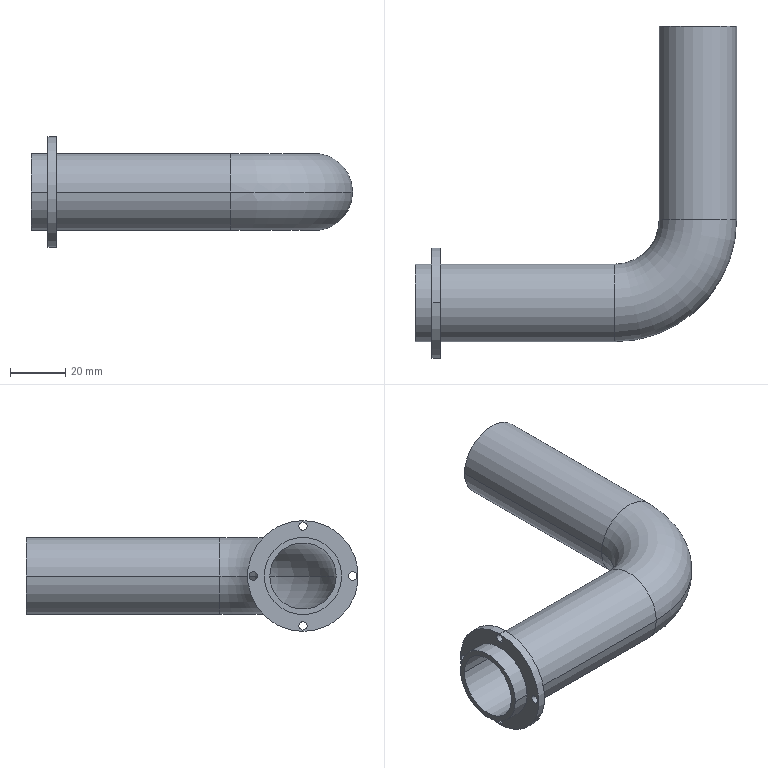Part | SolidWorks | features ICE 1, Shell 1, Sweep 1 | 1 solid | 28 faces | box 116 x 120 x 40 mm | volume 32734 mm3 | cylinder 20 | torus 4 | plane 4 | commonest cylinder face diameters 3 x8 28 x6 24 x4 40 x2
STEP:
#1=CARTESIAN_POINT('',(-12.,-70.,0.));
#2=VERTEX_POINT('',#1);
#3=CARTESIAN_POINT('',(12.,-70.,0.));
#4=VERTEX_POINT('',#3);
#5=CARTESIAN_POINT('',(0.,-70.,0.));
#6=DIRECTION('',(0.,1.,0.));
#7=DIRECTION('',(1.,0.,0.));
#8=AXIS2_PLACEMENT_3D('',#5,#6,#7);
#9=CIRCLE('',#8,12.);
#10=EDGE_CURVE('',#2,#4,#9,.T.);
#11=ORIENTED_EDGE('',*,*,#10,.T.);
#12=CARTESIAN_POINT('',(-30.,-112.,0.));
#13=VERTEX_POINT('',#12);
#14=CARTESIAN_POINT('',(-30.,-70.,0.));
#15=DIRECTION('',(0.,0.,-1.));
#16=DIRECTION('',(-1.,0.,0.));
#17=AXIS2_PLACEMENT_3D('',#14,#15,#16);
#18=CIRCLE('',#17,42.);
#19=EDGE_CURVE('',#4,#13,#18,.T.);
#20=ORIENTED_EDGE('',*,*,#19,.T.);
#21=CARTESIAN_POINT('',(-30.,-88.,0.));
#22=VERTEX_POINT('',#21);
#23=CARTESIAN_POINT('',(-30.,-100.,0.));
#24=DIRECTION('',(1.,0.,0.));
#25=DIRECTION('',(0.,1.,0.));
#26=AXIS2_PLACEMENT_3D('',#23,#24,#25);
#27=CIRCLE('',#26,12.);
#28=EDGE_CURVE('',#22,#13,#27,.T.);
#29=ORIENTED_EDGE('',*,*,#28,.F.);
#30=CARTESIAN_POINT('',(-30.,-70.,0.));
#31=DIRECTION('',(0.,0.,-1.));
#32=DIRECTION('',(-1.,0.,0.));
#33=AXIS2_PLACEMENT_3D('',#30,#31,#32);
#34=CIRCLE('',#33,18.);
#35=EDGE_CURVE('',#2,#22,#34,.T.);
#36=ORIENTED_EDGE('',*,*,#35,.F.);
#37=EDGE_LOOP('',(#11,#20,#29,#36));
#38=FACE_OUTER_BOUND('',#37,.T.);
#39=CARTESIAN_POINT('',(-30.,-70.,0.));
#40=DIRECTION('',(0.,0.,-1.));
#41=DIRECTION('',(-1.,0.,0.));
#42=AXIS2_PLACEMENT_3D('',#39,#40,#41);
#43=TOROIDAL_SURFACE('',#42,30.,12.);
#44=ADVANCED_FACE('',(#38),#43,.F.);
#45=CARTESIAN_POINT('',(14.,-70.,0.));
#46=VERTEX_POINT('',#45);
#47=CARTESIAN_POINT('',(-14.,-70.,0.));
#48=VERTEX_POINT('',#47);
#49=CARTESIAN_POINT('',(0.,-70.,0.));
#50=DIRECTION('',(0.,1.,0.));
#51=DIRECTION('',(0.,0.,-1.));
#52=AXIS2_PLACEMENT_3D('',#49,#50,#51);
#53=CIRCLE('',#52,14.);
#54=EDGE_CURVE('',#46,#48,#53,.T.);
#55=ORIENTED_EDGE('',*,*,#54,.F.);
#56=CARTESIAN_POINT('',(-30.,-114.,0.));
#57=VERTEX_POINT('',#56);
#58=CARTESIAN_POINT('',(-30.,-70.,0.));
#59=DIRECTION('',(0.,0.,-1.));
#60=DIRECTION('',(-1.,0.,0.));
#61=AXIS2_PLACEMENT_3D('',#58,#59,#60);
#62=CIRCLE('',#61,44.);
#63=EDGE_CURVE('',#46,#57,#62,.T.);
#64=ORIENTED_EDGE('',*,*,#63,.T.);
#65=CARTESIAN_POINT('',(-30.,-86.,0.));
#66=VERTEX_POINT('',#65);
#67=CARTESIAN_POINT('',(-30.,-100.,0.));
#68=DIRECTION('',(1.,0.,0.));
#69=DIRECTION('',(0.,0.,-1.));
#70=AXIS2_PLACEMENT_3D('',#67,#68,#69);
#71=CIRCLE('',#70,14.);
#72=EDGE_CURVE('',#57,#66,#71,.T.);
#73=ORIENTED_EDGE('',*,*,#72,.T.);
#74=CARTESIAN_POINT('',(-30.,-70.,0.));
#75=DIRECTION('',(0.,0.,-1.));
#76=DIRECTION('',(-1.,0.,0.));
#77=AXIS2_PLACEMENT_3D('',#74,#75,#76);
#78=CIRCLE('',#77,16.);
#79=EDGE_CURVE('',#48,#66,#78,.T.);
#80=ORIENTED_EDGE('',*,*,#79,.F.);
#81=EDGE_LOOP('',(#55,#64,#73,#80));
#82=FACE_OUTER_BOUND('',#81,.T.);
#83=CARTESIAN_POINT('',(-30.,-70.,0.));
#84=DIRECTION('',(0.,0.,-1.));
#85=DIRECTION('',(-1.,0.,0.));
#86=AXIS2_PLACEMENT_3D('',#83,#84,#85);
#87=TOROIDAL_SURFACE('',#86,30.,14.);
#88=ADVANCED_FACE('',(#82),#87,.T.);
#89=CARTESIAN_POINT('',(-93.,-100.,-19.5));
#90=VERTEX_POINT('',#89);
#91=CARTESIAN_POINT('',(-93.,-100.,-16.5));
#92=VERTEX_POINT('',#91);
#93=CARTESIAN_POINT('',(-93.,-100.,-18.));
#94=DIRECTION('',(-1.,0.,0.));
#95=DIRECTION('',(0.,0.,1.));
#96=AXIS2_PLACEMENT_3D('',#93,#94,#95);
#97=CIRCLE('',#96,1.5);
#98=EDGE_CURVE('',#90,#92,#97,.T.);
#99=ORIENTED_EDGE('',*,*,#98,.F.);
#100=CARTESIAN_POINT('',(-96.,-100.,-19.5));
#101=VERTEX_POINT('',#100);
#102=CARTESIAN_POINT('',(-93.,-100.,-19.5));
#103=DIRECTION('',(-1.,0.,0.));
#104=VECTOR('',#103,1000.);
#105=LINE('',#102,#104);
#106=EDGE_CURVE('',#90,#101,#105,.T.);
#107=ORIENTED_EDGE('',*,*,#106,.T.);
#108=CARTESIAN_POINT('',(-96.,-100.,-16.5));
#109=VERTEX_POINT('',#108);
#110=CARTESIAN_POINT('',(-96.,-100.,-18.));
#111=DIRECTION('',(-1.,0.,0.));
#112=DIRECTION('',(0.,0.,1.));
#113=AXIS2_PLACEMENT_3D('',#110,#111,#112);
#114=CIRCLE('',#113,1.5);
#115=EDGE_CURVE('',#101,#109,#114,.T.);
#116=ORIENTED_EDGE('',*,*,#115,.T.);
#117=CARTESIAN_POINT('',(-93.,-100.,-16.5));
#118=DIRECTION('',(-1.,0.,0.));
#119=VECTOR('',#118,1000.);
#120=LINE('',#117,#119);
#121=EDGE_CURVE('',#92,#109,#120,.T.);
#122=ORIENTED_EDGE('',*,*,#121,.F.);
#123=EDGE_LOOP('',(#99,#107,#116,#122));
#124=FACE_OUTER_BOUND('',#123,.T.);
#125=CARTESIAN_POINT('',(-93.,-100.,-18.));
#126=DIRECTION('',(-1.,0.,0.));
#127=DIRECTION('',(0.,0.,1.));
#128=AXIS2_PLACEMENT_3D('',#125,#126,#127);
#129=CYLINDRICAL_SURFACE('',#128,1.5);
#130=ADVANCED_FACE('',(#124),#129,.F.);
#131=CARTESIAN_POINT('',(-93.,-118.,-1.5));
#132=VERTEX_POINT('',#131);
#133=CARTESIAN_POINT('',(-93.,-118.,1.5));
#134=VERTEX_POINT('',#133);
#135=CARTESIAN_POINT('',(-93.,-118.,0.));
#136=DIRECTION('',(-1.,0.,0.));
#137=DIRECTION('',(0.,0.,1.));
#138=AXIS2_PLACEMENT_3D('',#135,#136,#137);
#139=CIRCLE('',#138,1.5);
#140=EDGE_CURVE('',#132,#134,#139,.T.);
#141=ORIENTED_EDGE('',*,*,#140,.F.);
#142=CARTESIAN_POINT('',(-96.,-118.,-1.5));
#143=VERTEX_POINT('',#142);
#144=CARTESIAN_POINT('',(-93.,-118.,-1.5));
#145=DIRECTION('',(-1.,0.,0.));
#146=VECTOR('',#145,1000.);
#147=LINE('',#144,#146);
#148=EDGE_CURVE('',#132,#143,#147,.T.);
#149=ORIENTED_EDGE('',*,*,#148,.T.);
#150=CARTESIAN_POINT('',(-96.,-118.,1.5));
#151=VERTEX_POINT('',#150);
#152=CARTESIAN_POINT('',(-96.,-118.,0.));
#153=DIRECTION('',(-1.,0.,0.));
#154=DIRECTION('',(0.,0.,1.));
#155=AXIS2_PLACEMENT_3D('',#152,#153,#154);
#156=CIRCLE('',#155,1.5);
#157=EDGE_CURVE('',#143,#151,#156,.T.);
#158=ORIENTED_EDGE('',*,*,#157,.T.);
#159=CARTESIAN_POINT('',(-93.,-118.,1.5));
#160=DIRECTION('',(-1.,0.,0.));
#161=VECTOR('',#160,1000.);
#162=LINE('',#159,#161);
#163=EDGE_CURVE('',#134,#151,#162,.T.);
#164=ORIENTED_EDGE('',*,*,#163,.F.);
#165=EDGE_LOOP('',(#141,#149,#158,#164));
#166=FACE_OUTER_BOUND('',#165,.T.);
#167=CARTESIAN_POINT('',(-93.,-118.,0.));
#168=DIRECTION('',(-1.,0.,0.));
#169=DIRECTION('',(0.,0.,1.));
#170=AXIS2_PLACEMENT_3D('',#167,#168,#169);
#171=CYLINDRICAL_SURFACE('',#170,1.5);
#172=ADVANCED_FACE('',(#166),#171,.F.);
#173=CARTESIAN_POINT('',(-93.,-100.,16.5));
#174=VERTEX_POINT('',#173);
#175=CARTESIAN_POINT('',(-93.,-100.,19.5));
#176=VERTEX_POINT('',#175);
#177=CARTESIAN_POINT('',(-93.,-100.,18.));
#178=DIRECTION('',(-1.,0.,0.));
#179=DIRECTION('',(0.,0.,1.));
#180=AXIS2_PLACEMENT_3D('',#177,#178,#179);
#181=CIRCLE('',#180,1.5);
#182=EDGE_CURVE('',#174,#176,#181,.T.);
#183=ORIENTED_EDGE('',*,*,#182,.F.);
#184=CARTESIAN_POINT('',(-96.,-100.,16.5));
#185=VERTEX_POINT('',#184);
#186=CARTESIAN_POINT('',(-93.,-100.,16.5));
#187=DIRECTION('',(-1.,0.,0.));
#188=VECTOR('',#187,1000.);
#189=LINE('',#186,#188);
#190=EDGE_CURVE('',#174,#185,#189,.T.);
#191=ORIENTED_EDGE('',*,*,#190,.T.);
#192=CARTESIAN_POINT('',(-96.,-100.,19.5));
#193=VERTEX_POINT('',#192);
#194=CARTESIAN_POINT('',(-96.,-100.,18.));
#195=DIRECTION('',(-1.,0.,0.));
#196=DIRECTION('',(0.,0.,1.));
#197=AXIS2_PLACEMENT_3D('',#194,#195,#196);
#198=CIRCLE('',#197,1.5);
#199=EDGE_CURVE('',#185,#193,#198,.T.);
#200=ORIENTED_EDGE('',*,*,#199,.T.);
#201=CARTESIAN_POINT('',(-93.,-100.,19.5));
#202=DIRECTION('',(-1.,0.,0.));
#203=VECTOR('',#202,1000.);
#204=LINE('',#201,#203);
#205=EDGE_CURVE('',#176,#193,#204,.T.);
#206=ORIENTED_EDGE('',*,*,#205,.F.);
#207=EDGE_LOOP('',(#183,#191,#200,#206));
#208=FACE_OUTER_BOUND('',#207,.T.);
#209=CARTESIAN_POINT('',(-93.,-100.,18.));
#210=DIRECTION('',(-1.,0.,0.));
#211=DIRECTION('',(0.,0.,1.));
#212=AXIS2_PLACEMENT_3D('',#209,#210,#211);
#213=CYLINDRICAL_SURFACE('',#212,1.5);
#214=ADVANCED_FACE('',(#208),#213,.F.);
#215=CARTESIAN_POINT('',(-93.,-82.,-1.5));
#216=VERTEX_POINT('',#215);
#217=CARTESIAN_POINT('',(-93.,-82.,1.5));
#218=VERTEX_POINT('',#217);
#219=CARTESIAN_POINT('',(-93.,-82.,0.));
#220=DIRECTION('',(-1.,0.,0.));
#221=DIRECTION('',(0.,0.,1.));
#222=AXIS2_PLACEMENT_3D('',#219,#220,#221);
#223=CIRCLE('',#222,1.5);
#224=EDGE_CURVE('',#216,#218,#223,.T.);
#225=ORIENTED_EDGE('',*,*,#224,.F.);
#226=CARTESIAN_POINT('',(-96.,-82.,-1.5));
#227=VERTEX_POINT('',#226);
#228=CARTESIAN_POINT('',(-93.,-82.,-1.5));
#229=DIRECTION('',(-1.,0.,0.));
#230=VECTOR('',#229,1000.);
#231=LINE('',#228,#230);
#232=EDGE_CURVE('',#216,#227,#231,.T.);
#233=ORIENTED_EDGE('',*,*,#232,.T.);
#234=CARTESIAN_POINT('',(-96.,-82.,1.5));
#235=VERTEX_POINT('',#234);
#236=CARTESIAN_POINT('',(-96.,-82.,0.));
#237=DIRECTION('',(-1.,0.,0.));
#238=DIRECTION('',(0.,0.,1.));
#239=AXIS2_PLACEMENT_3D('',#236,#237,#238);
#240=CIRCLE('',#239,1.5);
#241=EDGE_CURVE('',#227,#235,#240,.T.);
#242=ORIENTED_EDGE('',*,*,#241,.T.);
#243=CARTESIAN_POINT('',(-93.,-82.,1.5));
#244=DIRECTION('',(-1.,0.,0.));
#245=VECTOR('',#244,1000.);
#246=LINE('',#243,#245);
#247=EDGE_CURVE('',#218,#235,#246,.T.);
#248=ORIENTED_EDGE('',*,*,#247,.F.);
#249=EDGE_LOOP('',(#225,#233,#242,#248));
#250=FACE_OUTER_BOUND('',#249,.T.);
#251=CARTESIAN_POINT('',(-93.,-82.,0.));
#252=DIRECTION('',(-1.,0.,0.));
#253=DIRECTION('',(0.,0.,1.));
#254=AXIS2_PLACEMENT_3D('',#251,#252,#253);
#255=CYLINDRICAL_SURFACE('',#254,1.5);
#256=ADVANCED_FACE('',(#250),#255,.F.);
#257=CARTESIAN_POINT('',(-93.,-100.,20.));
#258=VERTEX_POINT('',#257);
#259=CARTESIAN_POINT('',(-93.,-100.,-20.));
#260=VERTEX_POINT('',#259);
#261=CARTESIAN_POINT('',(-93.,-100.,0.));
#262=DIRECTION('',(-1.,0.,0.));
#263=DIRECTION('',(0.,0.,1.));
#264=AXIS2_PLACEMENT_3D('',#261,#262,#263);
#265=CIRCLE('',#264,20.);
#266=EDGE_CURVE('',#258,#260,#265,.T.);
#267=ORIENTED_EDGE('',*,*,#266,.T.);
#268=CARTESIAN_POINT('',(-96.,-100.,-20.));
#269=VERTEX_POINT('',#268);
#270=CARTESIAN_POINT('',(-93.,-100.,-20.));
#271=DIRECTION('',(-1.,0.,0.));
#272=VECTOR('',#271,1000.);
#273=LINE('',#270,#272);
#274=EDGE_CURVE('',#260,#269,#273,.T.);
#275=ORIENTED_EDGE('',*,*,#274,.T.);
#276=CARTESIAN_POINT('',(-96.,-100.,20.));
#277=VERTEX_POINT('',#276);
#278=CARTESIAN_POINT('',(-96.,-100.,0.));
#279=DIRECTION('',(-1.,0.,0.));
#280=DIRECTION('',(0.,0.,1.));
#281=AXIS2_PLACEMENT_3D('',#278,#279,#280);
#282=CIRCLE('',#281,20.);
#283=EDGE_CURVE('',#277,#269,#282,.T.);
#284=ORIENTED_EDGE('',*,*,#283,.F.);
#285=CARTESIAN_POINT('',(-93.,-100.,20.));
#286=DIRECTION('',(-1.,0.,0.));
#287=VECTOR('',#286,1000.);
#288=LINE('',#285,#287);
#289=EDGE_CURVE('',#258,#277,#288,.T.);
#290=ORIENTED_EDGE('',*,*,#289,.F.);
#291=EDGE_LOOP('',(#267,#275,#284,#290));
#292=FACE_OUTER_BOUND('',#291,.T.);
#293=CARTESIAN_POINT('',(-93.,-100.,0.));
#294=DIRECTION('',(-1.,0.,0.));
#295=DIRECTION('',(0.,0.,1.));
#296=AXIS2_PLACEMENT_3D('',#293,#294,#295);
#297=CYLINDRICAL_SURFACE('',#296,20.);
#298=ADVANCED_FACE('',(#292),#297,.T.);
#299=CARTESIAN_POINT('',(-30.,-100.,0.));
#300=DIRECTION('',(1.,0.,0.));
#301=DIRECTION('',(0.,1.,0.));
#302=AXIS2_PLACEMENT_3D('',#299,#300,#301);
#303=CIRCLE('',#302,12.);
#304=EDGE_CURVE('',#13,#22,#303,.T.);
#305=ORIENTED_EDGE('',*,*,#304,.T.);
#306=CARTESIAN_POINT('',(-102.,-88.,0.));
#307=VERTEX_POINT('',#306);
#308=CARTESIAN_POINT('',(-30.,-88.,0.));
#309=DIRECTION('',(-1.,0.,0.));
#310=VECTOR('',#309,1000.);
#311=LINE('',#308,#310);
#312=EDGE_CURVE('',#22,#307,#311,.T.);
#313=ORIENTED_EDGE('',*,*,#312,.T.);
#314=CARTESIAN_POINT('',(-102.,-112.,0.));
#315=VERTEX_POINT('',#314);
#316=CARTESIAN_POINT('',(-102.,-100.,0.));
#317=DIRECTION('',(1.,0.,0.));
#318=DIRECTION('',(0.,0.,-1.));
#319=AXIS2_PLACEMENT_3D('',#316,#317,#318);
#320=CIRCLE('',#319,12.);
#321=EDGE_CURVE('',#315,#307,#320,.T.);
#322=ORIENTED_EDGE('',*,*,#321,.F.);
#323=CARTESIAN_POINT('',(-30.,-112.,0.));
#324=DIRECTION('',(-1.,0.,0.));
#325=VECTOR('',#324,1000.);
#326=LINE('',#323,#325);
#327=EDGE_CURVE('',#13,#315,#326,.T.);
#328=ORIENTED_EDGE('',*,*,#327,.F.);
#329=EDGE_LOOP('',(#305,#313,#322,#328));
#330=FACE_OUTER_BOUND('',#329,.T.);
#331=CARTESIAN_POINT('',(-30.,-100.,0.));
#332=DIRECTION('',(-1.,0.,0.));
#333=DIRECTION('',(0.,-1.,0.));
#334=AXIS2_PLACEMENT_3D('',#331,#332,#333);
#335=CYLINDRICAL_SURFACE('',#334,12.);
#336=ADVANCED_FACE('',(#330),#335,.F.);
#337=CARTESIAN_POINT('',(12.,0.,0.));
#338=VERTEX_POINT('',#337);
#339=CARTESIAN_POINT('',(-12.,0.,0.));
#340=VERTEX_POINT('',#339);
#341=CARTESIAN_POINT('',(0.,0.,0.));
#342=DIRECTION('',(0.,1.,0.));
#343=DIRECTION('',(-1.,0.,0.));
#344=AXIS2_PLACEMENT_3D('',#341,#342,#343);
#345=CIRCLE('',#344,12.);
#346=EDGE_CURVE('',#338,#340,#345,.T.);
#347=ORIENTED_EDGE('',*,*,#346,.T.);
#348=CARTESIAN_POINT('',(-12.,0.,0.));
#349=DIRECTION('',(0.,-1.,0.));
#350=VECTOR('',#349,1000.);
#351=LINE('',#348,#350);
#352=EDGE_CURVE('',#340,#2,#351,.T.);
#353=ORIENTED_EDGE('',*,*,#352,.T.);
#354=CARTESIAN_POINT('',(0.,-70.,0.));
#355=DIRECTION('',(0.,1.,0.));
#356=DIRECTION('',(1.,0.,0.));
#357=AXIS2_PLACEMENT_3D('',#354,#355,#356);
#358=CIRCLE('',#357,12.);
#359=EDGE_CURVE('',#4,#2,#358,.T.);
#360=ORIENTED_EDGE('',*,*,#359,.F.);
#361=CARTESIAN_POINT('',(12.,0.,0.));
#362=DIRECTION('',(0.,-1.,0.));
#363=VECTOR('',#362,1000.);
#364=LINE('',#361,#363);
#365=EDGE_CURVE('',#338,#4,#364,.T.);
#366=ORIENTED_EDGE('',*,*,#365,.F.);
#367=EDGE_LOOP('',(#347,#353,#360,#366));
#368=FACE_OUTER_BOUND('',#367,.T.);
#369=CARTESIAN_POINT('',(0.,0.,0.));
#370=DIRECTION('',(0.,-1.,0.));
#371=DIRECTION('',(1.,0.,0.));
#372=AXIS2_PLACEMENT_3D('',#369,#370,#371);
#373=CYLINDRICAL_SURFACE('',#372,12.);
#374=ADVANCED_FACE('',(#368),#373,.F.);
#375=CARTESIAN_POINT('',(-96.,-114.,0.));
#376=VERTEX_POINT('',#375);
#377=CARTESIAN_POINT('',(-96.,-86.,0.));
#378=VERTEX_POINT('',#377);
#379=CARTESIAN_POINT('',(-96.,-100.,0.));
#380=DIRECTION('',(-1.,0.,0.));
#381=DIRECTION('',(0.,0.,1.));
#382=AXIS2_PLACEMENT_3D('',#379,#380,#381);
#383=CIRCLE('',#382,14.);
#384=EDGE_CURVE('',#376,#378,#383,.T.);
#385=ORIENTED_EDGE('',*,*,#384,.T.);
#386=CARTESIAN_POINT('',(-102.,-86.,0.));
#387=VERTEX_POINT('',#386);
#388=CARTESIAN_POINT('',(-30.,-86.,0.));
#389=DIRECTION('',(-1.,0.,0.));
#390=VECTOR('',#389,1000.);
#391=LINE('',#388,#390);
#392=EDGE_CURVE('',#378,#387,#391,.T.);
#393=ORIENTED_EDGE('',*,*,#392,.T.);
#394=CARTESIAN_POINT('',(-102.,-114.,0.));
#395=VERTEX_POINT('',#394);
#396=CARTESIAN_POINT('',(-102.,-100.,0.));
#397=DIRECTION('',(1.,0.,0.));
#398=DIRECTION('',(0.,0.,-1.));
#399=AXIS2_PLACEMENT_3D('',#396,#397,#398);
#400=CIRCLE('',#399,14.);
#401=EDGE_CURVE('',#387,#395,#400,.T.);
#402=ORIENTED_EDGE('',*,*,#401,.T.);
#403=CARTESIAN_POINT('',(-30.,-114.,0.));
#404=DIRECTION('',(-1.,0.,0.));
#405=VECTOR('',#404,1000.);
#406=LINE('',#403,#405);
#407=EDGE_CURVE('',#376,#395,#406,.T.);
#408=ORIENTED_EDGE('',*,*,#407,.F.);
#409=EDGE_LOOP('',(#385,#393,#402,#408));
#410=FACE_OUTER_BOUND('',#409,.T.);
#411=CARTESIAN_POINT('',(-30.,-100.,0.));
#412=DIRECTION('',(-1.,0.,0.));
#413=DIRECTION('',(0.,-1.,0.));
#414=AXIS2_PLACEMENT_3D('',#411,#412,#413);
#415=CYLINDRICAL_SURFACE('',#414,14.);
#416=ADVANCED_FACE('',(#410),#415,.T.);
#417=CARTESIAN_POINT('',(-14.,0.,0.));
#418=VERTEX_POINT('',#417);
#419=CARTESIAN_POINT('',(14.,0.,0.));
#420=VERTEX_POINT('',#419);
#421=CARTESIAN_POINT('',(0.,0.,0.));
#422=DIRECTION('',(0.,1.,0.));
#423=DIRECTION('',(0.,0.,-1.));
#424=AXIS2_PLACEMENT_3D('',#421,#422,#423);
#425=CIRCLE('',#424,14.);
#426=EDGE_CURVE('',#418,#420,#425,.T.);
#427=ORIENTED_EDGE('',*,*,#426,.F.);
#428=CARTESIAN_POINT('',(-14.,0.,0.));
#429=DIRECTION('',(0.,-1.,0.));
#430=VECTOR('',#429,1000.);
#431=LINE('',#428,#430);
#432=EDGE_CURVE('',#418,#48,#431,.T.);
#433=ORIENTED_EDGE('',*,*,#432,.T.);
#434=CARTESIAN_POINT('',(0.,-70.,0.));
#435=DIRECTION('',(0.,1.,0.));
#436=DIRECTION('',(0.,0.,-1.));
#437=AXIS2_PLACEMENT_3D('',#434,#435,#436);
#438=CIRCLE('',#437,14.);
#439=EDGE_CURVE('',#48,#46,#438,.T.);
#440=ORIENTED_EDGE('',*,*,#439,.T.);
#441=CARTESIAN_POINT('',(14.,0.,0.));
#442=DIRECTION('',(0.,-1.,0.));
#443=VECTOR('',#442,1000.);
#444=LINE('',#441,#443);
#445=EDGE_CURVE('',#420,#46,#444,.T.);
#446=ORIENTED_EDGE('',*,*,#445,.F.);
#447=EDGE_LOOP('',(#427,#433,#440,#446));
#448=FACE_OUTER_BOUND('',#447,.T.);
#449=CARTESIAN_POINT('',(0.,0.,0.));
#450=DIRECTION('',(0.,-1.,0.));
#451=DIRECTION('',(1.,0.,0.));
#452=AXIS2_PLACEMENT_3D('',#449,#450,#451);
#453=CYLINDRICAL_SURFACE('',#452,14.);
#454=ADVANCED_FACE('',(#448),#453,.T.);
#455=CARTESIAN_POINT('',(-30.,-100.,0.));
#456=DIRECTION('',(1.,0.,0.));
#457=DIRECTION('',(0.,0.,-1.));
#458=AXIS2_PLACEMENT_3D('',#455,#456,#457);
#459=CIRCLE('',#458,14.);
#460=EDGE_CURVE('',#66,#57,#459,.T.);
#461=ORIENTED_EDGE('',*,*,#460,.F.);
#462=CARTESIAN_POINT('',(-93.,-86.,0.));
#463=VERTEX_POINT('',#462);
#464=CARTESIAN_POINT('',(-30.,-86.,0.));
#465=DIRECTION('',(-1.,0.,0.));
#466=VECTOR('',#465,1000.);
#467=LINE('',#464,#466);
#468=EDGE_CURVE('',#66,#463,#467,.T.);
#469=ORIENTED_EDGE('',*,*,#468,.T.);
#470=CARTESIAN_POINT('',(-93.,-114.,0.));
#471=VERTEX_POINT('',#470);
#472=CARTESIAN_POINT('',(-93.,-100.,0.));
#473=DIRECTION('',(-1.,0.,0.));
#474=DIRECTION('',(0.,0.,1.));
#475=AXIS2_PLACEMENT_3D('',#472,#473,#474);
#476=CIRCLE('',#475,14.);
#477=EDGE_CURVE('',#471,#463,#476,.T.);
#478=ORIENTED_EDGE('',*,*,#477,.F.);
#479=CARTESIAN_POINT('',(-30.,-114.,0.));
#480=DIRECTION('',(-1.,0.,0.));
#481=VECTOR('',#480,1000.);
#482=LINE('',#479,#481);
#483=EDGE_CURVE('',#57,#471,#482,.T.);
#484=ORIENTED_EDGE('',*,*,#483,.F.);
#485=EDGE_LOOP('',(#461,#469,#478,#484));
#486=FACE_OUTER_BOUND('',#485,.T.);
#487=CARTESIAN_POINT('',(-30.,-100.,0.));
#488=DIRECTION('',(-1.,0.,0.));
#489=DIRECTION('',(0.,-1.,0.));
#490=AXIS2_PLACEMENT_3D('',#487,#488,#489);
#491=CYLINDRICAL_SURFACE('',#490,14.);
#492=ADVANCED_FACE('',(#486),#491,.T.);
#493=ORIENTED_EDGE('',*,*,#468,.F.);
#494=ORIENTED_EDGE('',*,*,#72,.F.);
#495=ORIENTED_EDGE('',*,*,#483,.T.);
#496=CARTESIAN_POINT('',(-93.,-100.,0.));
#497=DIRECTION('',(-1.,0.,0.));
#498=DIRECTION('',(0.,0.,1.));
#499=AXIS2_PLACEMENT_3D('',#496,#497,#498);
#500=CIRCLE('',#499,14.);
#501=EDGE_CURVE('',#463,#471,#500,.T.);
#502=ORIENTED_EDGE('',*,*,#501,.F.);
#503=EDGE_LOOP('',(#493,#494,#495,#502));
#504=FACE_OUTER_BOUND('',#503,.T.);
#505=CARTESIAN_POINT('',(-30.,-100.,0.));
#506=DIRECTION('',(-1.,0.,0.));
#507=DIRECTION('',(0.,-1.,0.));
#508=AXIS2_PLACEMENT_3D('',#505,#506,#507);
#509=CYLINDRICAL_SURFACE('',#508,14.);
#510=ADVANCED_FACE('',(#504),#509,.T.);
#511=ORIENTED_EDGE('',*,*,#392,.F.);
#512=CARTESIAN_POINT('',(-96.,-100.,0.));
#513=DIRECTION('',(-1.,0.,0.));
#514=DIRECTION('',(0.,0.,1.));
#515=AXIS2_PLACEMENT_3D('',#512,#513,#514);
#516=CIRCLE('',#515,14.);
#517=EDGE_CURVE('',#378,#376,#516,.T.);
#518=ORIENTED_EDGE('',*,*,#517,.T.);
#519=ORIENTED_EDGE('',*,*,#407,.T.);
#520=CARTESIAN_POINT('',(-102.,-100.,0.));
#521=DIRECTION('',(1.,0.,0.));
#522=DIRECTION('',(0.,0.,-1.));
#523=AXIS2_PLACEMENT_3D('',#520,#521,#522);
#524=CIRCLE('',#523,14.);
#525=EDGE_CURVE('',#395,#387,#524,.T.);
#526=ORIENTED_EDGE('',*,*,#525,.T.);
#527=EDGE_LOOP('',(#511,#518,#519,#526));
#528=FACE_OUTER_BOUND('',#527,.T.);
#529=CARTESIAN_POINT('',(-30.,-100.,0.));
#530=DIRECTION('',(-1.,0.,0.));
#531=DIRECTION('',(0.,-1.,0.));
#532=AXIS2_PLACEMENT_3D('',#529,#530,#531);
#533=CYLINDRICAL_SURFACE('',#532,14.);
#534=ADVANCED_FACE('',(#528),#533,.T.);
#535=ORIENTED_EDGE('',*,*,#63,.F.);
#536=ORIENTED_EDGE('',*,*,#439,.F.);
#537=ORIENTED_EDGE('',*,*,#79,.T.);
#538=ORIENTED_EDGE('',*,*,#460,.T.);
#539=EDGE_LOOP('',(#535,#536,#537,#538));
#540=FACE_OUTER_BOUND('',#539,.T.);
#541=CARTESIAN_POINT('',(-30.,-70.,0.));
#542=DIRECTION('',(0.,0.,-1.));
#543=DIRECTION('',(-1.,0.,0.));
#544=AXIS2_PLACEMENT_3D('',#541,#542,#543);
#545=TOROIDAL_SURFACE('',#544,30.,14.);
#546=ADVANCED_FACE('',(#540),#545,.T.);
#547=ORIENTED_EDGE('',*,*,#432,.F.);
#548=CARTESIAN_POINT('',(0.,0.,0.));
#549=DIRECTION('',(0.,1.,0.));
#550=DIRECTION('',(0.,0.,-1.));
#551=AXIS2_PLACEMENT_3D('',#548,#549,#550);
#552=CIRCLE('',#551,14.);
#553=EDGE_CURVE('',#420,#418,#552,.T.);
#554=ORIENTED_EDGE('',*,*,#553,.F.);
#555=ORIENTED_EDGE('',*,*,#445,.T.);
#556=ORIENTED_EDGE('',*,*,#54,.T.);
#557=EDGE_LOOP('',(#547,#554,#555,#556));
#558=FACE_OUTER_BOUND('',#557,.T.);
#559=CARTESIAN_POINT('',(0.,0.,0.));
#560=DIRECTION('',(0.,-1.,0.));
#561=DIRECTION('',(1.,0.,0.));
#562=AXIS2_PLACEMENT_3D('',#559,#560,#561);
#563=CYLINDRICAL_SURFACE('',#562,14.);
#564=ADVANCED_FACE('',(#558),#563,.T.);
#565=ORIENTED_EDGE('',*,*,#321,.T.);
#566=CARTESIAN_POINT('',(-102.,-100.,0.));
#567=DIRECTION('',(1.,0.,0.));
#568=DIRECTION('',(0.,0.,-1.));
#569=AXIS2_PLACEMENT_3D('',#566,#567,#568);
#570=CIRCLE('',#569,12.);
#571=EDGE_CURVE('',#307,#315,#570,.T.);
#572=ORIENTED_EDGE('',*,*,#571,.T.);
#573=EDGE_LOOP('',(#565,#572));
#574=FACE_BOUND('',#573,.T.);
#575=ORIENTED_EDGE('',*,*,#525,.F.);
#576=ORIENTED_EDGE('',*,*,#401,.F.);
#577=EDGE_LOOP('',(#575,#576));
#578=FACE_OUTER_BOUND('',#577,.T.);
#579=CARTESIAN_POINT('',(-102.,-100.,0.));
#580=DIRECTION('',(1.,0.,0.));
#581=DIRECTION('',(0.,0.,-1.));
#582=AXIS2_PLACEMENT_3D('',#579,#580,#581);
#583=PLANE('',#582);
#584=ADVANCED_FACE('',(#574,#578),#583,.F.);
#585=ORIENTED_EDGE('',*,*,#346,.F.);
#586=CARTESIAN_POINT('',(0.,0.,0.));
#587=DIRECTION('',(0.,1.,0.));
#588=DIRECTION('',(-1.,0.,0.));
#589=AXIS2_PLACEMENT_3D('',#586,#587,#588);
#590=CIRCLE('',#589,12.);
#591=EDGE_CURVE('',#340,#338,#590,.T.);
#592=ORIENTED_EDGE('',*,*,#591,.F.);
#593=EDGE_LOOP('',(#585,#592));
#594=FACE_BOUND('',#593,.T.);
#595=ORIENTED_EDGE('',*,*,#553,.T.);
#596=ORIENTED_EDGE('',*,*,#426,.T.);
#597=EDGE_LOOP('',(#595,#596));
#598=FACE_OUTER_BOUND('',#597,.T.);
#599=CARTESIAN_POINT('',(0.,0.,0.));
#600=DIRECTION('',(0.,1.,0.));
#601=DIRECTION('',(0.,0.,-1.));
#602=AXIS2_PLACEMENT_3D('',#599,#600,#601);
#603=PLANE('',#602);
#604=ADVANCED_FACE('',(#594,#598),#603,.T.);
#605=ORIENTED_EDGE('',*,*,#312,.F.);
#606=ORIENTED_EDGE('',*,*,#28,.T.);
#607=ORIENTED_EDGE('',*,*,#327,.T.);
#608=ORIENTED_EDGE('',*,*,#571,.F.);
#609=EDGE_LOOP('',(#605,#606,#607,#608));
#610=FACE_OUTER_BOUND('',#609,.T.);
#611=CARTESIAN_POINT('',(-30.,-100.,0.));
#612=DIRECTION('',(-1.,0.,0.));
#613=DIRECTION('',(0.,-1.,0.));
#614=AXIS2_PLACEMENT_3D('',#611,#612,#613);
#615=CYLINDRICAL_SURFACE('',#614,12.);
#616=ADVANCED_FACE('',(#610),#615,.F.);
#617=ORIENTED_EDGE('',*,*,#19,.F.);
#618=ORIENTED_EDGE('',*,*,#359,.T.);
#619=ORIENTED_EDGE('',*,*,#35,.T.);
#620=ORIENTED_EDGE('',*,*,#304,.F.);
#621=EDGE_LOOP('',(#617,#618,#619,#620));
#622=FACE_OUTER_BOUND('',#621,.T.);
#623=CARTESIAN_POINT('',(-30.,-70.,0.));
#624=DIRECTION('',(0.,0.,-1.));
#625=DIRECTION('',(-1.,0.,0.));
#626=AXIS2_PLACEMENT_3D('',#623,#624,#625);
#627=TOROIDAL_SURFACE('',#626,30.,12.);
#628=ADVANCED_FACE('',(#622),#627,.F.);
#629=ORIENTED_EDGE('',*,*,#352,.F.);
#630=ORIENTED_EDGE('',*,*,#591,.T.);
#631=ORIENTED_EDGE('',*,*,#365,.T.);
#632=ORIENTED_EDGE('',*,*,#10,.F.);
#633=EDGE_LOOP('',(#629,#630,#631,#632));
#634=FACE_OUTER_BOUND('',#633,.T.);
#635=CARTESIAN_POINT('',(0.,0.,0.));
#636=DIRECTION('',(0.,-1.,0.));
#637=DIRECTION('',(1.,0.,0.));
#638=AXIS2_PLACEMENT_3D('',#635,#636,#637);
#639=CYLINDRICAL_SURFACE('',#638,12.);
#640=ADVANCED_FACE('',(#634),#639,.F.);
#641=ORIENTED_EDGE('',*,*,#266,.F.);
#642=CARTESIAN_POINT('',(-93.,-100.,0.));
#643=DIRECTION('',(-1.,0.,0.));
#644=DIRECTION('',(0.,0.,1.));
#645=AXIS2_PLACEMENT_3D('',#642,#643,#644);
#646=CIRCLE('',#645,20.);
#647=EDGE_CURVE('',#260,#258,#646,.T.);
#648=ORIENTED_EDGE('',*,*,#647,.F.);
#649=EDGE_LOOP('',(#641,#648));
#650=FACE_OUTER_BOUND('',#649,.T.);
#651=CARTESIAN_POINT('',(-93.,-82.,0.));
#652=DIRECTION('',(-1.,0.,0.));
#653=DIRECTION('',(0.,0.,1.));
#654=AXIS2_PLACEMENT_3D('',#651,#652,#653);
#655=CIRCLE('',#654,1.5);
#656=EDGE_CURVE('',#218,#216,#655,.T.);
#657=ORIENTED_EDGE('',*,*,#656,.T.);
#658=ORIENTED_EDGE('',*,*,#224,.T.);
#659=EDGE_LOOP('',(#657,#658));
#660=FACE_BOUND('',#659,.T.);
#661=CARTESIAN_POINT('',(-93.,-100.,18.));
#662=DIRECTION('',(-1.,0.,0.));
#663=DIRECTION('',(0.,0.,1.));
#664=AXIS2_PLACEMENT_3D('',#661,#662,#663);
#665=CIRCLE('',#664,1.5);
#666=EDGE_CURVE('',#176,#174,#665,.T.);
#667=ORIENTED_EDGE('',*,*,#666,.T.);
#668=ORIENTED_EDGE('',*,*,#182,.T.);
#669=EDGE_LOOP('',(#667,#668));
#670=FACE_BOUND('',#669,.T.);
#671=CARTESIAN_POINT('',(-93.,-118.,0.));
#672=DIRECTION('',(-1.,0.,0.));
#673=DIRECTION('',(0.,0.,1.));
#674=AXIS2_PLACEMENT_3D('',#671,#672,#673);
#675=CIRCLE('',#674,1.5);
#676=EDGE_CURVE('',#134,#132,#675,.T.);
#677=ORIENTED_EDGE('',*,*,#676,.T.);
#678=ORIENTED_EDGE('',*,*,#140,.T.);
#679=EDGE_LOOP('',(#677,#678));
#680=FACE_BOUND('',#679,.T.);
#681=CARTESIAN_POINT('',(-93.,-100.,-18.));
#682=DIRECTION('',(-1.,0.,0.));
#683=DIRECTION('',(0.,0.,1.));
#684=AXIS2_PLACEMENT_3D('',#681,#682,#683);
#685=CIRCLE('',#684,1.5);
#686=EDGE_CURVE('',#92,#90,#685,.T.);
#687=ORIENTED_EDGE('',*,*,#686,.T.);
#688=ORIENTED_EDGE('',*,*,#98,.T.);
#689=EDGE_LOOP('',(#687,#688));
#690=FACE_BOUND('',#689,.T.);
#691=ORIENTED_EDGE('',*,*,#477,.T.);
#692=ORIENTED_EDGE('',*,*,#501,.T.);
#693=EDGE_LOOP('',(#691,#692));
#694=FACE_BOUND('',#693,.T.);
#695=CARTESIAN_POINT('',(-93.,-100.,0.));
#696=DIRECTION('',(-1.,0.,0.));
#697=DIRECTION('',(0.,0.,1.));
#698=AXIS2_PLACEMENT_3D('',#695,#696,#697);
#699=PLANE('',#698);
#700=ADVANCED_FACE('',(#650,#660,#670,#680,#690,#694),#699,.F.);
#701=ORIENTED_EDGE('',*,*,#283,.T.);
#702=CARTESIAN_POINT('',(-96.,-100.,0.));
#703=DIRECTION('',(-1.,0.,0.));
#704=DIRECTION('',(0.,0.,1.));
#705=AXIS2_PLACEMENT_3D('',#702,#703,#704);
#706=CIRCLE('',#705,20.);
#707=EDGE_CURVE('',#269,#277,#706,.T.);
#708=ORIENTED_EDGE('',*,*,#707,.T.);
#709=EDGE_LOOP('',(#701,#708));
#710=FACE_OUTER_BOUND('',#709,.T.);
#711=CARTESIAN_POINT('',(-96.,-82.,0.));
#712=DIRECTION('',(-1.,0.,0.));
#713=DIRECTION('',(0.,0.,1.));
#714=AXIS2_PLACEMENT_3D('',#711,#712,#713);
#715=CIRCLE('',#714,1.5);
#716=EDGE_CURVE('',#235,#227,#715,.T.);
#717=ORIENTED_EDGE('',*,*,#716,.F.);
#718=ORIENTED_EDGE('',*,*,#241,.F.);
#719=EDGE_LOOP('',(#717,#718));
#720=FACE_BOUND('',#719,.T.);
#721=CARTESIAN_POINT('',(-96.,-100.,18.));
#722=DIRECTION('',(-1.,0.,0.));
#723=DIRECTION('',(0.,0.,1.));
#724=AXIS2_PLACEMENT_3D('',#721,#722,#723);
#725=CIRCLE('',#724,1.5);
#726=EDGE_CURVE('',#193,#185,#725,.T.);
#727=ORIENTED_EDGE('',*,*,#726,.F.);
#728=ORIENTED_EDGE('',*,*,#199,.F.);
#729=EDGE_LOOP('',(#727,#728));
#730=FACE_BOUND('',#729,.T.);
#731=CARTESIAN_POINT('',(-96.,-118.,0.));
#732=DIRECTION('',(-1.,0.,0.));
#733=DIRECTION('',(0.,0.,1.));
#734=AXIS2_PLACEMENT_3D('',#731,#732,#733);
#735=CIRCLE('',#734,1.5);
#736=EDGE_CURVE('',#151,#143,#735,.T.);
#737=ORIENTED_EDGE('',*,*,#736,.F.);
#738=ORIENTED_EDGE('',*,*,#157,.F.);
#739=EDGE_LOOP('',(#737,#738));
#740=FACE_BOUND('',#739,.T.);
#741=CARTESIAN_POINT('',(-96.,-100.,-18.));
#742=DIRECTION('',(-1.,0.,0.));
#743=DIRECTION('',(0.,0.,1.));
#744=AXIS2_PLACEMENT_3D('',#741,#742,#743);
#745=CIRCLE('',#744,1.5);
#746=EDGE_CURVE('',#109,#101,#745,.T.);
#747=ORIENTED_EDGE('',*,*,#746,.F.);
#748=ORIENTED_EDGE('',*,*,#115,.F.);
#749=EDGE_LOOP('',(#747,#748));
#750=FACE_BOUND('',#749,.T.);
#751=ORIENTED_EDGE('',*,*,#384,.F.);
#752=ORIENTED_EDGE('',*,*,#517,.F.);
#753=EDGE_LOOP('',(#751,#752));
#754=FACE_BOUND('',#753,.T.);
#755=CARTESIAN_POINT('',(-96.,-100.,0.));
#756=DIRECTION('',(-1.,0.,0.));
#757=DIRECTION('',(0.,0.,1.));
#758=AXIS2_PLACEMENT_3D('',#755,#756,#757);
#759=PLANE('',#758);
#760=ADVANCED_FACE('',(#710,#720,#730,#740,#750,#754),#759,.T.);
#761=ORIENTED_EDGE('',*,*,#274,.F.);
#762=ORIENTED_EDGE('',*,*,#647,.T.);
#763=ORIENTED_EDGE('',*,*,#289,.T.);
#764=ORIENTED_EDGE('',*,*,#707,.F.);
#765=EDGE_LOOP('',(#761,#762,#763,#764));
#766=FACE_OUTER_BOUND('',#765,.T.);
#767=CARTESIAN_POINT('',(-93.,-100.,0.));
#768=DIRECTION('',(-1.,0.,0.));
#769=DIRECTION('',(0.,0.,1.));
#770=AXIS2_PLACEMENT_3D('',#767,#768,#769);
#771=CYLINDRICAL_SURFACE('',#770,20.);
#772=ADVANCED_FACE('',(#766),#771,.T.);
#773=ORIENTED_EDGE('',*,*,#232,.F.);
#774=ORIENTED_EDGE('',*,*,#656,.F.);
#775=ORIENTED_EDGE('',*,*,#247,.T.);
#776=ORIENTED_EDGE('',*,*,#716,.T.);
#777=EDGE_LOOP('',(#773,#774,#775,#776));
#778=FACE_OUTER_BOUND('',#777,.T.);
#779=CARTESIAN_POINT('',(-93.,-82.,0.));
#780=DIRECTION('',(-1.,0.,0.));
#781=DIRECTION('',(0.,0.,1.));
#782=AXIS2_PLACEMENT_3D('',#779,#780,#781);
#783=CYLINDRICAL_SURFACE('',#782,1.5);
#784=ADVANCED_FACE('',(#778),#783,.F.);
#785=ORIENTED_EDGE('',*,*,#190,.F.);
#786=ORIENTED_EDGE('',*,*,#666,.F.);
#787=ORIENTED_EDGE('',*,*,#205,.T.);
#788=ORIENTED_EDGE('',*,*,#726,.T.);
#789=EDGE_LOOP('',(#785,#786,#787,#788));
#790=FACE_OUTER_BOUND('',#789,.T.);
#791=CARTESIAN_POINT('',(-93.,-100.,18.));
#792=DIRECTION('',(-1.,0.,0.));
#793=DIRECTION('',(0.,0.,1.));
#794=AXIS2_PLACEMENT_3D('',#791,#792,#793);
#795=CYLINDRICAL_SURFACE('',#794,1.5);
#796=ADVANCED_FACE('',(#790),#795,.F.);
#797=ORIENTED_EDGE('',*,*,#148,.F.);
#798=ORIENTED_EDGE('',*,*,#676,.F.);
#799=ORIENTED_EDGE('',*,*,#163,.T.);
#800=ORIENTED_EDGE('',*,*,#736,.T.);
#801=EDGE_LOOP('',(#797,#798,#799,#800));
#802=FACE_OUTER_BOUND('',#801,.T.);
#803=CARTESIAN_POINT('',(-93.,-118.,0.));
#804=DIRECTION('',(-1.,0.,0.));
#805=DIRECTION('',(0.,0.,1.));
#806=AXIS2_PLACEMENT_3D('',#803,#804,#805);
#807=CYLINDRICAL_SURFACE('',#806,1.5);
#808=ADVANCED_FACE('',(#802),#807,.F.);
#809=ORIENTED_EDGE('',*,*,#106,.F.);
#810=ORIENTED_EDGE('',*,*,#686,.F.);
#811=ORIENTED_EDGE('',*,*,#121,.T.);
#812=ORIENTED_EDGE('',*,*,#746,.T.);
#813=EDGE_LOOP('',(#809,#810,#811,#812));
#814=FACE_OUTER_BOUND('',#813,.T.);
#815=CARTESIAN_POINT('',(-93.,-100.,-18.));
#816=DIRECTION('',(-1.,0.,0.));
#817=DIRECTION('',(0.,0.,1.));
#818=AXIS2_PLACEMENT_3D('',#815,#816,#817);
#819=CYLINDRICAL_SURFACE('',#818,1.5);
#820=ADVANCED_FACE('',(#814),#819,.F.);
#821=CLOSED_SHELL('',(#44,#88,#130,#172,#214,#256,#298,#336,#374,#416,#454,#492,#510,#534,#546,#564,#584,#604,#616,#628,#640,#700,#760,#772,#784,#796,#808,#820));
#822=MANIFOLD_SOLID_BREP('',#821);
#823=CARTESIAN_POINT('',(0.,0.,0.));
#824=DIRECTION('',(0.,0.,1.));
#825=DIRECTION('',(1.,0.,0.));
#826=AXIS2_PLACEMENT_3D('',#823,#824,#825);
#827=(LENGTH_UNIT()NAMED_UNIT(*)SI_UNIT(.MILLI.,.METRE.));
#828=UNCERTAINTY_MEASURE_WITH_UNIT(LENGTH_MEASURE(0.00001),#827,'','');
#829=(NAMED_UNIT(*)PLANE_ANGLE_UNIT()SI_UNIT($,.RADIAN.));
#830=(NAMED_UNIT(*)SI_UNIT($,.STERADIAN.)SOLID_ANGLE_UNIT());
#831=(GEOMETRIC_REPRESENTATION_CONTEXT(3)GLOBAL_UNCERTAINTY_ASSIGNED_CONTEXT((#828))GLOBAL_UNIT_ASSIGNED_CONTEXT((#827,#829,#830))REPRESENTATION_CONTEXT('',''));
#832=ADVANCED_BREP_SHAPE_REPRESENTATION('',(#822,#826),#831);